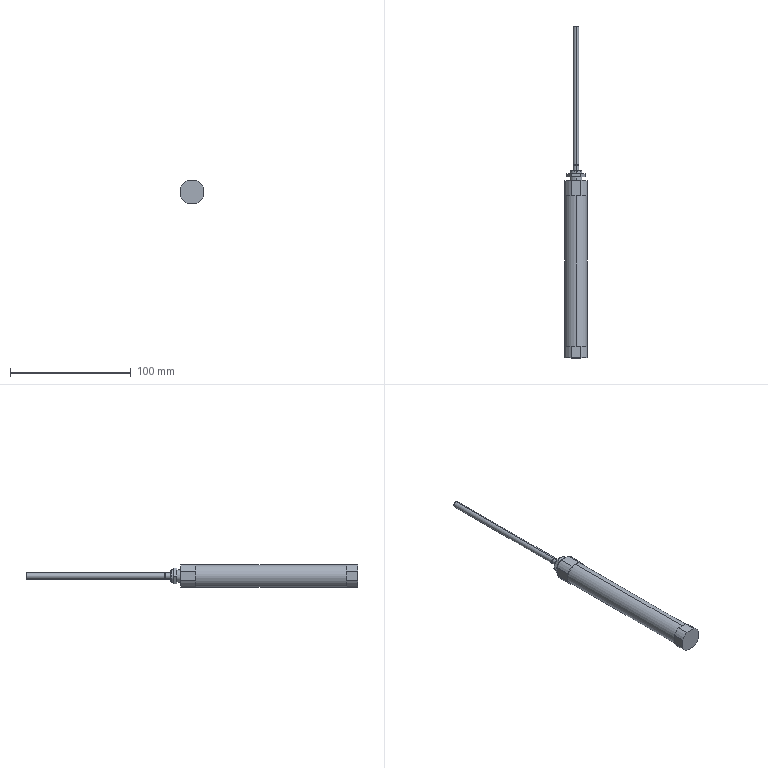Part | SolidWorks | features ICE 6, Chamfer 3, Extrusion 1, HoleWzd 1 | 1 solid | 61 faces | box 18.3 x 275 x 18.3 mm | volume 42130 mm3 | plane 29 | cylinder 22 | cone 10 | commonest cylinder face diameters 20 x8 4.2 x4 5 x4 10 x4 18.3 x2